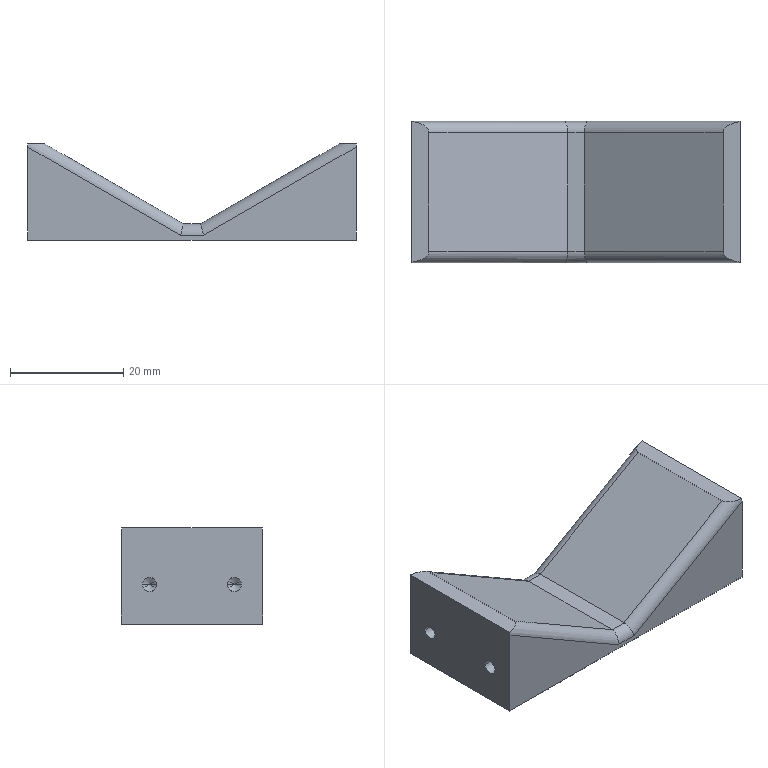Part | 1 solid | 56 faces | box 58 x 25 x 17 mm | volume 14370 mm3 | cylinder 30 | cone 16 | plane 10 | commonest cylinder face diameters 2.5 x16 3.3 x8 4 x6